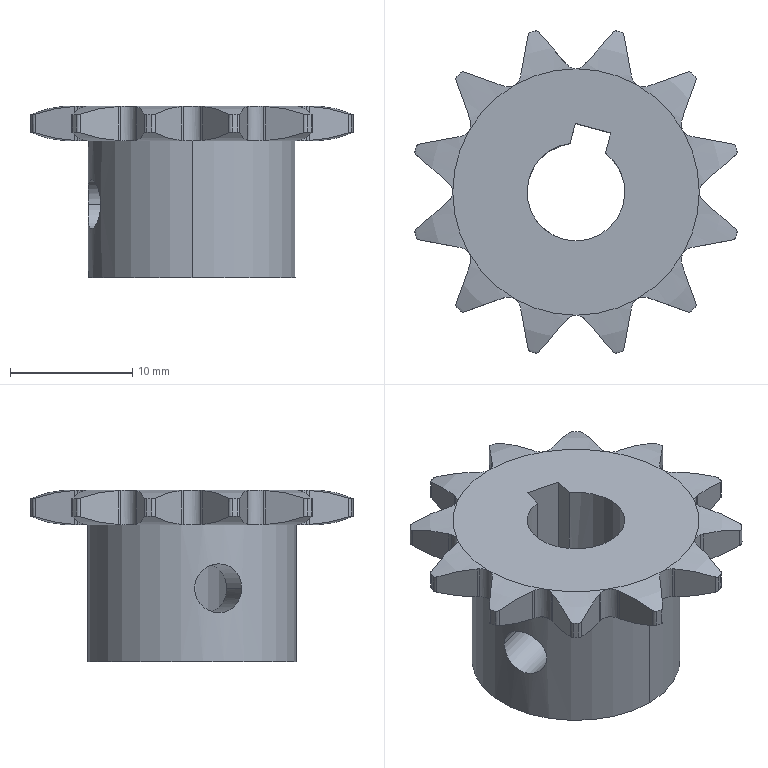Part | SolidWorks | features MBimport 1 | 1 solid | 137 faces | box 26.325 x 26.325 x 14 mm | volume 2835 mm3 | cylinder 80 | plane 33 | torus 24 | commonest cylinder face diameters 0.6 x24 8.78 x24 2 x12 27.13 x12 4 x4 8 x2